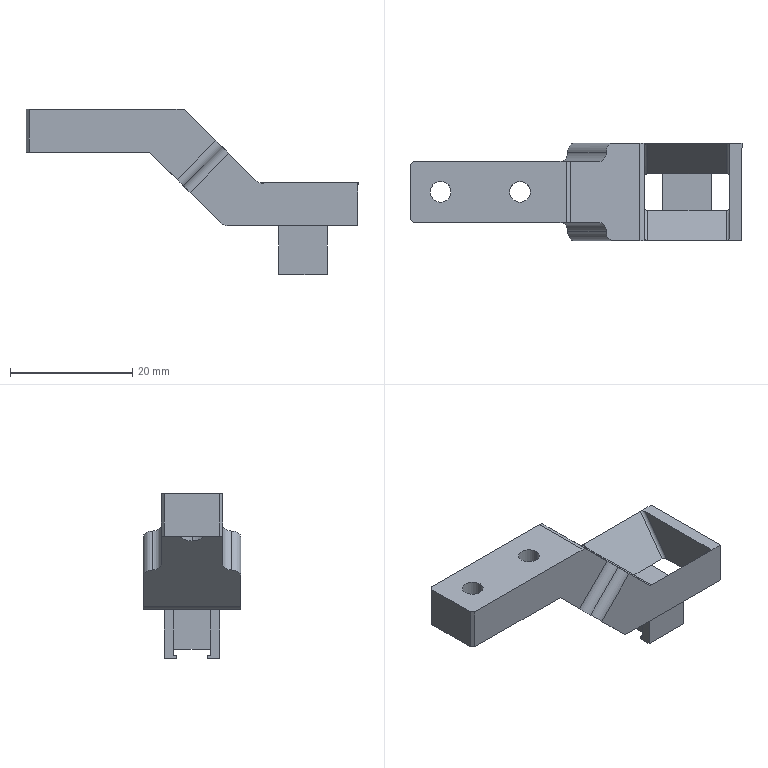NC program | NX | posted with a generic post | part box 54.3 x 16 x 27 mm
Lines 1 to 2092 of 2256, first 1710 of 2082 lines:
N10 G17 G21 G94 G90
(FLOOR_WALL_COPY , TOOL : D63)
N12 T01 M6
N14 G54
N16 G17 G0 G90 X61.65 Y0. S6500 M3
N18 G43 Z30. H1
N20 Z5.
N22 G94 G1 Z2. F1250.
N24 X58.65
N26 X-58.65
N28 X-61.65
N30 Z5.
N32 G0 Z30.
N34 X61.65
N36 Z4.
N38 G1 Z1.
N40 X58.65
N42 X-58.65
N44 X-61.65
N46 Z4.
N48 G0 Z30.
N50 X61.65
N52 Z3.
N54 G1 Z0.
N56 X58.65
N58 X-58.65
N60 X-61.65
N62 Z3.
N64 G0 Z30.
N66 M5
(ADAPTIVE_MILLING_COPY , TOOL : D10)
N68 T10 M6
N70 G54
N72 G17 G0 G90 X-34.694 Y5.359 S9500 M3
N74 G43 Z30. H10
N76 Z-19.
N78 G94 G1 Z-20. F1000.
N80 X-33.303 Y5.066 F3000.
N82 G3 X-32.119 Y5.793 R1.015
N84 G2 X-30.91 Y8.416 R7.757
N86 X-26.126 Y11.331 R8.866
N88 X-19.787 Y12.096 R28.107
N90 X-3.589 Y12.207 R872.404
N92 X-1.666 Y12.973 R40.193
N94 G3 X-1.294 Y14.73 R1.002
N96 X-2.022 Y14.954 Z-19.961 R1.2
N98 G1 X-3.242 Y15.048 Z-19.9
N100 X-5.564 Y15.223
N102 X-18.689
N104 G3 X-27.308 Y14.162 R35.782
N106 G1 X-29.988 Y13.492
N108 G3 X-32.384 Y11.72 R3.927
N110 G1 X-33.273 Y10.231
N112 X-33.344 Y9.998
N114 X-33.595 Y8.591
N116 X-33.946 Y6.622 Z-20.
N118 G3 X-32.052 Y5.992 R1.001
N120 G1 X-31.586 Y7.089
N122 X-31.512 Y7.213
N124 G2 X-29.711 Y9.133 R10.188
N126 X-27.095 Y10.189 R7.286
N128 X-18.08 Y11.276 R40.593
N130 X-5.381 Y11.398 R731.827
N132 G3 X-4.212 Y11.674 R2.037
N134 G1 X-3.221 Y12.351
N136 G3 X-2.96 Y13.916 R1.104
N138 X-4.038 Y14.346 Z-19.939 R1.126
N140 G1 X-4.815 Y14.276 Z-19.9
N142 X-22.927 Y12.645
N144 X-24.919 Y12.466 Z-20.
N146 X-28.102 Y12.179
N148 G3 X-27.771 Y10.008 R-1.1
N150 G2 X-24.571 Y10.157 R20.137
N152 X-7.279 Y10.583 R306.496
N154 G3 X-5.015 Y10.897 R6.389
N156 X-4.229 Y11.659 R4.398
N158 X-4.031 Y13.088 R1.106
N160 X-5.114 Y13.579 Z-19.937 R1.124
N162 G1 X-5.858 Y13.533 Z-19.9
N164 X-20.163 Y12.646
N166 X-22.16 Y12.522 Z-20.
N168 X-25.039 Y12.343
N170 G3 X-24.971 Y10.145 R1.1
N172 G1 X-6.671 Y10.15
N174 X-6.571 Y10.152
N176 X-6.471 Y10.156
N178 X-6.371 Y10.162
N180 X-6.271 Y10.171
N182 G3 X-5.5 Y10.363 R3.095
N184 X-6.169 Y12.398 R1.101
N186 G1 X-6.941 Y12.316
N188 G3 X-6.671 Y10.15 R1.1
N190 X-5.187 Y10.618 R1.697
N192 G1 X-4.784 Y11.062
N194 G3 X-4.802 Y12.436 R1.015
N196 G1 X-5.859 Y13.547
N198 Z-17.
N200 G0 Z30.
N202 X-1.019 Y-15.568
N204 Z-19.
N206 G1 Z-20. F1000.
N208 X-0.945 Y-14.723 F3000.
N210 X-0.895 Y-13.875
N212 G3 X-1.673 Y-12.97 R1.017
N214 X-5.422 Y-12.354 R12.902
N216 X-17.32 Y-12.208 R274.583
N218 G2 X-25.019 Y-12.171 R212.132
N220 X-28.946 Y-9.646 R5.945
N222 G3 X-29.801 Y-9.066 R5.743
N224 G2 X-31.587 Y-7.088 R10.217
N226 G1 X-32.091 Y-5.9
N228 X-32.128 Y-5.76
N230 G3 X-34.083 Y-6.168 R1.
N232 G1 X-34.065 Y-6.286
N234 X-33.768 Y-8.264 Z-19.9
N236 X-33.664 Y-8.985
N238 X-33.539 Y-9.703
N240 X-33.437 Y-9.918
N242 X-33.293 Y-10.107
N244 X-31.166 Y-12.22
N246 G3 X-27.018 Y-14.768 R12.966
N248 X-25.001 Y-15.159 R7.211
N250 G1 X-5.151 Y-16.046
N252 X-4.921 Y-16.026
N254 X-4.7 Y-15.961
N256 X-2.947 Y-15.181
N258 X-2.346 Y-14.919 Z-19.933
N260 X-1.755 Y-14.634 Z-19.966
N262 G3 X-1.354 Y-14.092 Z-20. R1.039
N264 X-1.969 Y-12.864 R1.005
N266 X-4.395 Y-12.014 R21.801
N268 X-10.463 Y-11.485 R33.858
N270 G1 X-11.163 Y-11.47
N272 X-11.963 Y-11.456
N274 X-12.863 Y-11.445
N276 X-13.963 Y-11.436
N278 X-15.363 Y-11.428
N280 X-17.163 Y-11.422
N282 X-19.863 Y-11.418
N284 X-21.663 Y-11.416
N286 X-21.863 Y-11.414
N288 X-22.062 Y-11.407
N290 X-22.162 Y-11.401
N292 X-22.262 Y-11.394
N294 X-22.362 Y-11.386
N296 G2 X-26.048 Y-10.189 R10.868
N298 G1 X-26.145 Y-10.164
N300 X-26.244 Y-10.148
N302 X-26.273 Y-10.145
N304 X-26.571
N306 X-26.626 Y-10.142
N308 X-27.663 Y-10.031
N310 X-27.771 Y-10.008
N312 G2 X-29.181 Y-9.443 R5.526
N314 G3 X-29.862 Y-11.485 R-1.1
N316 G1 X-21.677 Y-12.417
N318 X-19.69 Y-12.644 Z-19.9
N320 X-4.721 Y-14.349
N322 X-4.174 Y-14.415 Z-19.928
N324 X-3.625 Y-14.459 Z-19.955
N326 G3 X-2.842 Y-14.073 Z-20. R1.127
N328 X-3.067 Y-12.447 R1.103
N330 X-6.588 Y-11.131 R7.515
N332 X-14.667 Y-10.662 R58.746
N334 G2 X-20.565 Y-10.571 R130.429
N336 X-22.98 Y-10.146 R25.993
N338 G1 X-26.28 Y-10.145
N340 G3 X-26.366 Y-12.342 R1.1
N342 G1 X-24.497 Y-12.488
N344 X-22.503 Y-12.644 Z-19.9
N346 X-5.256 Y-13.996
N348 X-4.712 Y-14.042 Z-19.927
N350 X-4.166 Y-14.066 Z-19.955
N352 G3 X-3.392 Y-13.645 Z-20. R1.127
N354 X-3.648 Y-12.057 R1.104
N356 X-7.522 Y-10.439 R7.948
N358 G1 X-7.817 Y-10.387
N360 X-8.015 Y-10.355
N362 X-8.312 Y-10.311
N364 X-8.609 Y-10.27
N366 X-8.906 Y-10.233
N368 X-9.205 Y-10.198
N370 X-9.503 Y-10.167
N372 X-9.693 Y-10.149
N374 X-22.993 Y-10.146
N376 G3 X-23.067 Y-12.343 R1.1
N378 G1 X-20.592 Y-12.511
N380 X-18.596 Y-12.646 Z-19.9
N382 X-5.928 Y-13.502
N384 X-4.895 Y-13.56 Z-19.952
N386 G3 X-4.083 Y-13.098 Z-20. R1.117
N388 X-4.263 Y-11.63 R1.106
N390 X-6.784 Y-10.15 R4.657
N392 G1 X-9.784 Y-10.149
N394 G3 X-9.982 Y-12.331 R1.1
N396 G1 X-5.563 Y-13.141
N398 G3 X-4.552 Y-11.318 R1.101
N400 X-5.819 Y-10.211 R3.706
N402 G1 X-5.916 Y-10.184
N404 G3 X-6.916 Y-11.916 R1.418
N406 G1 Z-17.
N408 G0 Z30.
N410 X-6.091 Y-12.459
N412 Z-19.
N414 G1 Z-20. F1000.
N416 G3 X-5.091 Y-10.727 R1.068 F3000.
N418 X-6.174 Y-10.15 R1.435
N420 G1 X-6.874
N422 G3 X-7.874 Y-11.018 R1.015
N424 G1 X-8.105 Y-12.649
N426 Z-17.
N428 G0 Z30.
N430 X-6.845 Y-12.646
N432 Z-18.85
N434 G1 Z-19.85 F1000.
N436 X-6.621 Y-11.939 F3000.
N438 X-6.419 Y-11.227
N440 G3 X-7.293 Y-10.082 R1.014
N442 G2 X-9.133 Y-9.716 R13.216
N444 G3 X-15.616 Y-9.336 R44.907
N446 G1 X-16.615 Y-9.326
N448 X-17.715 Y-9.319
N450 X-19.415 Y-9.312
N452 X-21.715 Y-9.307
N454 X-23.815 Y-9.305
N456 X-24.115 Y-9.303
N458 X-24.315 Y-9.296
N460 X-24.515 Y-9.284
N462 X-24.615 Y-9.277
N464 G2 X-29.165 Y-6.37 R6.019
N466 X-30.957 Y-0.905 R12.945
N468 X-31.153 Y2.882 R17.934
N470 X-28.239 Y7.11 R6.115
N472 X-22.771 Y8.898 R13.157
N474 X-13.784 Y9.273 R80.836
N476 G3 X-9.687 Y9.319 R120.043
N478 G1 X-9.591 Y9.346
N480 X-9.497 Y9.381
N482 X-9.456 Y9.392
N484 X-9.406 Y9.429
N486 X-9.288 Y9.497
N488 X-8.163 Y9.955
N490 X-8.031 Y9.99
N492 X-7.336 Y10.077
N494 G3 X-7.266 Y12.05 R1.
N496 G1 X-9.26 Y12.195 Z-19.75
N498 X-11.233 Y12.327
N500 X-15.116 Y12.331
N502 X-18.998 Y12.315
N504 G3 X-24.303 Y11.742 R33.616
N506 G1 X-26.55 Y11.302
N508 G3 X-28.997 Y10.23 R8.544
N510 X-31.394 Y8.505 R21.965
N512 X-33.33 Y5.962 R7.81
N514 G1 X-34.047 Y4.412
N516 G3 X-34.505 Y1.269 R7.014
N518 X-33.857 Y-2.409 R21.764
N520 G1 X-33.058 Y-5.333
N522 G3 X-30.706 Y-9.442 R10.958
N524 X-27.868 Y-11.569 R11.21
N526 X-26.314 Y-12.061 R5.955
N528 G1 X-25.081 Y-12.23
N530 X-23.842 Y-12.343
N532 X-11.345 Y-13.137
N534 X-11.1 Y-13.119
N536 X-10.864 Y-13.048
N538 X-9.157 Y-12.264
N540 X-8.56 Y-11.996 Z-19.783
N542 X-7.973 Y-11.705 Z-19.816
N544 G3 X-7.579 Y-11.156 Z-19.85 R1.038
N546 X-8.163 Y-9.955 R1.005
N548 X-13.399 Y-8.727 R13.553
N550 X-22.095 Y-8.506 R179.279
N552 G2 X-28.226 Y-4.551 R7.728
N554 X-29.75 Y0.157 R9.996
N556 X-26.545 Y5.851 R6.994
N558 X-20.571 Y7.982 R13.882
N560 X-11.791 Y8.465 R72.135
N562 G3 X-10.334 Y8.726 R3.136
N564 G1 X-9.406 Y9.429
N566 G3 X-9.152 Y10.739 R1.005
N568 X-10.056 Y11.242 Z-19.796 R1.108
N570 G1 X-10.969 Y11.367 Z-19.75
N572 X-12.135 Y11.531
N574 X-13.303 Y11.679
N576 X-15.926 Y11.667
N578 G3 X-18.902 Y11.368 R23.497
N580 G1 X-21.305 Y10.971
N582 X-23.704 Y10.548
N584 G3 X-26.891 Y9.188 R10.193
N586 G1 X-27.71 Y8.621
N588 X-29.561 Y7.204
N590 G3 X-32.73 Y1.225 R9.176
N592 X-32.814 Y-1.042 R10.047
N594 X-31.855 Y-4.187 R8.525
N596 G1 X-31.089 Y-5.624
N598 X-30.306 Y-7.053
N600 G3 X-23.608 Y-11.372 R9.088
N602 G1 X-12.47 Y-12.679
N604 G3 X-11.896 Y-12.575 R1.05
N606 G1 X-10.355 Y-11.784
N608 X-9.763 Y-11.486 Z-19.783
N610 X-9.183 Y-11.166 Z-19.816
N612 G3 X-8.815 Y-10.617 Z-19.85 R1.04
N614 X-9.288 Y-9.497 R1.007
N616 X-12.559 Y-8.256 R7.076
N618 X-19.736 Y-7.767 R53.459
N620 G2 X-27.173 Y-3.154 R8.398
N622 X-25.88 Y3.62 R6.296
N624 X-20.28 Y6.732 R11.07
N626 X-13.542 Y7.556 R35.54
N628 G3 X-11.086 Y7.954 R8.006
N630 X-10.374 Y8.695 R3.575
N632 G1 X-10.294 Y8.756
N634 G3 X-10.025 Y10.039 R1.005
N636 X-10.85 Y10.556 Z-19.799 R1.036
N638 G1 X-11.825 Y10.7 Z-19.75
N640 X-12.933 Y10.87
N642 X-14.044 Y11.017
N644 X-14.191 Y11.006
N646 X-16.725 Y10.629
N648 X-19.255 Y10.231
N650 G3 X-23.855 Y8.721 R17.997
N652 G1 X-24.674 Y8.275
N654 X-25.468 Y7.786
N656 X-26.937 Y6.791
N658 G3 X-30.071 Y2.932 R9.819
N660 X-30.036 Y-4.241 R8.823
N662 X-29.08 Y-5.809 R8.521
N664 G1 X-28.315 Y-6.794
N666 X-27.518 Y-7.754
N668 G3 X-26.567 Y-8.544 R4.338
N670 G1 X-25.038 Y-9.453
N672 G3 X-22.043 Y-10.464 R9.838
N674 X-16.476 Y-11.211 R83.227
N676 G1 X-13.423 Y-11.502
N678 X-11.236 Y-11.196
N680 X-10.586 Y-11.109 Z-19.783
N682 X-9.94 Y-10.996 Z-19.816
N684 G3 X-9.407 Y-10.583 Z-19.85 R1.038
N686 X-9.645 Y-9.248 R1.005
N688 X-13.45 Y-7.57 R7.472
N690 X-18.618 Y-7.024 R54.385
N692 G2 X-23.16 Y-5.362 R8.744
N694 X-24.483 Y0.921 R5.298
N696 X-19.901 Y5.169 R8.486
N698 X-14.187 Y6.563 R22.236
N700 G3 X-11.583 Y7.227 R8.616
N702 X-10.787 Y8.193 R5.823
N704 X-10.704 Y9.294 R1.01
N706 X-11.429 Y9.8 Z-19.804 R1.05
N708 G1 X-12.482 Y10.065 Z-19.75
N710 X-13.363 Y10.291
N712 X-14.248 Y10.497
N714 X-14.468 Y10.491
N716 X-14.684 Y10.443
N718 G3 X-22.166 Y7.516 R103.306
N720 X-25.649 Y4.921 R11.193
N722 G1 X-26.749 Y3.678
N724 G3 X-27.894 Y1.069 R6.093
N726 X-28.036 Y-0.574 R8.104
N728 G1 X-27.976 Y-2.854
N730 G3 X-26.964 Y-5.913 R6.857
N732 X-25.992 Y-7.277 R8.317
N734 X-23.817 Y-8.745 R6.341
N736 G1 X-23.236 Y-8.958
N738 X-22.642 Y-9.13
N740 X-19.924 Y-9.778
N742 X-17.197 Y-10.386
N744 X-14.149 Y-10.961
N746 X-13.905 Y-10.946
N748 X-12.025 Y-10.599
N750 X-11.376 Y-10.484 Z-19.783
N752 X-10.731 Y-10.345 Z-19.816
N754 G3 X-10.218 Y-9.918 Z-19.85 R1.039
N756 X-10.374 Y-8.695 R1.007
N758 X-12.862 Y-7.221 R4.942
N760 X-17.477 Y-6.363 R33.121
N762 G2 X-20.725 Y-4.615 R4.609
N764 X-20.867 Y0.792 R5.115
N766 X-16.551 Y4.507 R8.832
N768 X-12.634 Y6.02 R423.42
N770 G3 X-11.582 Y6.817 R2.166
N772 G1 X-11.285 Y7.522
N774 X-11.235 Y7.609
N776 G3 X-11.352 Y8.781 R1.007
N778 X-12.261 Y9.105 Z-19.8 R1.037
N780 G1 X-13.254 Y9.042 Z-19.75
N782 X-15.116 Y8.923
N784 X-15.357 Y8.874
N786 X-15.581 Y8.773
N788 X-17.753 Y7.422
N790 X-19.916 Y6.056
N792 G3 X-22.572 Y3.943 R20.484
N794 X-24.39 Y0.271 R6.692
N796 X-24.365 Y-2.478 R8.177
N798 G1 X-24.214 Y-3.297
N800 X-24.013 Y-4.106
N802 G3 X-21.836 Y-7.454 R7.439
N804 X-18.412 Y-9.447 R9.742
N806 G1 X-14.43 Y-10.771
N808 G3 X-13.875 Y-10.793 R1.056
N810 G1 X-12.245 Y-10.391
N812 X-11.585 Y-10.233 Z-19.784
N814 X-10.931 Y-10.054 Z-19.818
N816 G3 X-10.457 Y-9.636 Z-19.85 R1.043
N818 X-10.532 Y-8.521 R1.01
N820 X-13.175 Y-6.65 R4.905
N822 G2 X-15.373 Y-5.98 R58.857
N824 X-17.484 Y-2.276 R3.983
N826 X-15.357 Y2.44 R6.994
N828 X-12.432 Y5.015 R49.357
N830 G3 X-11.793 Y6.271 R1.565
N832 G1 X-11.757 Y6.403
N834 X-11.563 Y6.864
N836 G3 X-11.966 Y8.107 R1.005
N838 X-12.933 Y8.151 Z-19.8 R1.037
N840 G1 X-13.86 Y7.798 Z-19.75
N842 X-14.853 Y7.423
N844 X-15.839 Y7.032
N846 X-16.063 Y6.864
N848 G3 X-17.105 Y5.709 R8.737
N850 G1 X-19.588 Y1.735
N852 G3 X-20.191 Y-2.998 R5.721
N854 G1 X-19.089 Y-6.475
N856 G3 X-16.905 Y-8.674 R3.401
N858 G1 X-15.155 Y-9.236
N860 X-12.948 Y-9.513
N862 X-12.296 Y-9.598 Z-19.783
N864 X-11.642 Y-9.659 Z-19.816
N866 G3 X-11.021 Y-9.403 Z-19.85 R1.039
N868 X-10.9 Y-8.047 R1.005
N870 X-12.642 Y-6.405 R5.646
N872 G2 X-14.353 Y-1.433 R5.328
N874 X-12.841 Y2.456 R10.733
N876 G3 X-11.994 Y4.04 R11.478
N878 G2 X-11.854 Y5.828 R15.376
N880 G3 X-13.091 Y6.934 R1.002
N882 X-13.775 Y6.381 Z-19.805 R1.172
N884 G1 X-14.41 Y5.487 Z-19.75
N886 X-15.672 Y3.71
N888 X-16.221 Y2.643
N890 X-16.718 Y1.551
N892 X-16.971 Y0.848
N894 X-17.186 Y0.133
N896 X-17.485 Y-0.991
N898 X-17.762 Y-2.12
N900 G3 X-16.984 Y-5.781 R4.962
N902 G1 X-15.716 Y-7.64
N904 G3 X-15.245 Y-8.012 R1.047
N906 G1 X-13.515 Y-8.669
N908 X-12.898 Y-8.909 Z-19.783
N910 X-12.273 Y-9.126 Z-19.816
N912 G3 X-11.617 Y-9.032 Z-19.85 R1.039
N914 X-11.216 Y-7.64 R1.004
N916 G2 X-12.271 Y-5.56 R22.33
N918 X-12.263 Y0.337 R9.427
N920 G3 X-11.942 Y1.595 R8.724
N922 G1 X-11.965 Y1.841
N924 X-11.968 Y1.891
N926 Y4.191
N928 G3 X-14.166 Y4.127 R-1.1
N930 G1 X-13.475 Y-7.829
N932 G3 X-11.363 Y-7.338 R-1.1
N934 G2 X-11.968 Y-4.964 R5.796
N936 X-11.891 Y-1.077 R35.506
N938 G3 X-11.706 Y0.223 R3.713
N940 G2 X-11.943 Y1.604 R11.623
N942 G3 X-12.978 Y2.517 R1.015
N944 G1 X-14.466 Y2.474
N946 Z-16.85
N948 G0 Z30.
N950 X-6.75 Y-12.611
N952 Z-17.806
N954 G1 Z-18.806 F1000.
N956 X-6.24 Y-12.163 F3000.
N958 X-5.748 Y-11.697
N960 G3 X-6.358 Y-10.076 R1.012
N962 G2 X-9.516 Y-8.488 R5.316
N964 X-10.937 Y-4.864 R5.696
N966 G1 X-10.942 Y-1.135
N968 G2 X-11.024 Y2.961 R35.702
N970 G3 X-10.926 Y5.036 R9.258
N972 G2 X-9.424 Y8.584 R5.579
N974 X-6.327 Y10.081 R5.365
N976 G3 X-5.89 Y11.852 R1.001
N978 X-6.511 Y12.083 Z-18.773 R1.287
N980 G1 X-7.818 Y12.325 Z-18.706
N982 X-8.654 Y12.487
N984 X-9.495 Y12.624
N986 G3 X-10.225 Y12.331 R1.026
N988 G1 X-11.236 Y11.324
N990 X-12.234 Y10.304
N992 G3 X-13.245 Y8.492 R5.115
N994 X-14.022 Y5.095 R21.177
N996 G1 X-14.086 Y4.351
N998 X-14.113 Y3.604
N1000 X-14.106 Y-1.9
N1002 X-14.05 Y-2.13
N1004 X-13.436 Y-3.783
N1006 X-12.819 Y-5.424 Z-18.794
N1008 X-12.68 Y-5.626 Z-18.806
N1010 G3 X-10.931 Y-4.963 R1.001
N1012 G1 Y3.565
N1014 G3 X-11.79 Y4.564 R1.016
N1016 G1 X-13.431 Y4.812
N1018 Z-15.806
N1020 G0 Z30.
N1022 X-6.587 Y-12.792
N1024 Z-17.21
N1026 G1 Z-18.21 F1000.
N1028 X-5.56 Y-11.727 F3000.
N1030 G3 X-5.977 Y-10.065 R1.012
N1032 G2 X-9.785 Y-7.279 R5.357
N1034 X-10.331 Y-4.968 R6.009
N1036 G1 Y4.986
N1038 X-10.327 Y5.048
N1040 G2 X-6.07 Y10.028 R5.166
N1042 G1 X-6.013 Y10.046
N1044 X-5.918 Y10.078
N1046 G3 X-5.517 Y11.732 R1.012
N1048 G1 X-6.567 Y12.829
N1050 Z-15.21
N1052 G0 Z30.
N1054 X-7.115 Y-11.501
N1056 Z-16.613
N1058 G1 Z-17.613 F1000.
N1060 G3 X-5.701 Y-10.087 R1.04 F3000.
N1062 G1 X-5.846 Y-10.004
N1064 X-7.12 Y-9.453
N1066 X-7.233 Y-9.387
N1068 G2 X-9.565 Y-6.254 R5.44
N1070 G1 X-9.726 Y-5.034
N1072 X-9.731 Y-4.965
N1074 Y4.965
N1076 X-9.726 Y5.035
N1078 G2 X-8.175 Y8.66 R5.519
N1080 X-5.92 Y9.979 R6.444
N1082 G3 X-5.777 Y11.756 R1.012
N1084 G1 X-6.896 Y12.473
N1086 Z-14.613
N1088 G0 Z30.
N1090 X-7.005 Y-11.472
N1092 Z-16.016
N1094 G1 Z-17.016 F1000.
N1096 G3 X-5.591 Y-10.058 R1.099 F3000.
N1098 X-6.976 Y-9.168 R6.404
N1100 G2 X-9.131 Y-4.969 R5.359
N1102 G1 Y4.969
N1104 X-9.127 Y5.031
N1106 G2 X-6.983 Y9.161 R5.307
N1108 G3 X-5.612 Y10.033 R6.372
N1110 G1 X-5.55 Y10.111
N1112 G3 X-5.698 Y11.511 R1.005
N1114 X-6.582 Y11.723 Z-16.969 R1.152
N1116 G1 X-7.644 Y11.661 Z-16.916
N1118 X-8.519 Y11.613
N1120 X-9.392 Y11.547
N1122 G3 X-9.897 Y11.275 R1.051
N1124 G1 X-10.293 Y10.881
N1126 X-10.657 Y10.458
N1128 X-10.849 Y10.143
N1130 X-11.009 Y9.81
N1132 X-11.776 Y7.82
N1134 G3 X-12.397 Y4.064 R11.823
N1136 G1 Y-7.022
N1138 G3 X-11.201 Y-9.937 R4.172
N1140 G1 X-10.556 Y-10.597
N1142 X-9.898 Y-11.244
N1144 G3 X-9.37 Y-11.444 R1.053
N1146 G1 X-7.879 Y-11.558
N1148 X-7.099 Y-11.62 Z-16.955
N1150 X-6.319 Y-11.666 Z-16.994
N1152 X-6.106 Y-11.624 Z-17.005
N1154 X-5.904 Y-11.544 Z-17.016
N1156 G3 X-5.802 Y-9.861 R1.001
N1158 X-7.331 Y-10.313 R1.013
N1160 G1 X-7.825 Y-11.573
N1162 Z-14.016
N1164 G0 Z30.
N1166 X-6.988 Y-12.335
N1168 Z-15.419
N1170 G1 Z-16.419 F1000.
N1172 X-5.798 Y-11.155 F3000.
N1174 G3 X-5.639 Y-9.925 R1.017
N1176 G1 X-5.69 Y-9.839
N1178 X-5.928 Y-9.517
N1180 X-5.994 Y-9.442
N1182 X-6.031 Y-9.405
N1184 G2 X-7.901 Y-7.438 R6.188
N1186 X-8.53 Y-4.966 R5.993
N1188 G1 Y4.966
N1190 X-8.526 Y5.034
N1192 G2 X-7.042 Y8.594 R5.493
N1194 G3 X-5.764 Y9.712 R7.285
N1196 G1 X-5.561 Y10.057
N1198 G3 X-5.997 Y11.469 R1.004
N1200 X-6.929 Y11.447 Z-16.371 R1.136
N1202 G1 X-7.908 Y11.106 Z-16.319
N1204 X-8.776 Y10.811
N1206 X-9.636 Y10.493
N1208 G3 X-10.061 Y10.057 R1.046
N1210 G1 X-10.794 Y8.565
N1212 G3 X-11.328 Y6.58 R7.405
N1214 X-11.699 Y2.357 R43.65
N1216 G1 X-11.709 Y1.359
N1218 X-11.698 Y0.362
N1220 X-11.514 Y-5.672
N1222 G3 X-10.803 Y-8.558 R7.18
N1224 G1 X-10.442 Y-9.314
N1226 X-10.059 Y-10.06
N1228 G3 X-9.566 Y-10.433 R1.044
N1230 G1 X-8.172 Y-10.914
N1232 X-7.432 Y-11.172 Z-16.359
N1234 X-6.687 Y-11.415 Z-16.398
N1236 X-6.472 Y-11.428 Z-16.409
N1238 X-6.258 Y-11.402 Z-16.419
N1240 G3 X-5.639 Y-9.925 R1.003
N1242 X-6.096 Y-9.352 R2.019
N1244 X-7.563 Y-9.571 R1.014
N1246 G1 X-8.362 Y-10.743
N1248 Z-13.419
N1250 G0 Z30.
N1252 X-7.5 Y-11.654
N1254 Z-14.823
N1256 G1 Z-15.823 F1000.
N1258 X-6.775 Y-11.153 F3000.
N1260 X-6.064 Y-10.632
N1262 G3 X-5.874 Y-9.437 R1.017
N1264 X-7.16 Y-7.676 R9.203
N1266 G2 X-7.93 Y-4.968 R5.773
N1268 G1 Y4.963
N1270 X-7.925 Y5.035
N1272 G2 X-7.198 Y7.612 R5.88
N1274 G1 X-7.119 Y7.738
N1276 X-6.213 Y8.808
N1278 X-6.075 Y9.017
N1280 X-5.807 Y9.554
N1282 G3 X-6.093 Y10.805 R1.017
N1284 G1 X-7.375 Y11.794
N1286 Z-12.823
N1288 G0 Z30.
N1290 X-7.908 Y-10.894
N1292 Z-14.226
N1294 G1 Z-15.226 F1000.
N1296 X-7.151 Y-10.491 F3000.
N1298 X-6.407 Y-10.067
N1300 G3 X-6.08 Y-8.904 R1.017
N1302 X-6.985 Y-6.883 R17.907
N1304 G2 X-7.33 Y-5.008 R6.062
N1306 G1 Y5.002
N1308 X-7.328 Y5.047
N1310 G2 X-6.507 Y7.86 R5.576
N1312 G1 X-6.05 Y8.969
N1314 G3 X-6.497 Y10.239 R1.015
N1316 G1 X-7.867 Y10.993
N1318 Z-12.226
N1320 G0 Z30.
N1322 X-8.312 Y-10.058
N1324 Z-13.629
N1326 G1 Z-14.629 F1000.
N1328 X-7.501 Y-9.72 F3000.
N1330 X-6.698 Y-9.36
N1332 G3 X-6.246 Y-8.28 R1.017
N1334 G2 X-6.73 Y-5.547 R12.969
N1336 G1 Y5.537
N1338 X-6.729 Y5.569
N1340 X-6.682 Y6.348
N1342 X-6.67 Y6.432
N1344 X-6.254 Y8.285
N1346 G3 X-6.848 Y9.438 R1.016
N1348 G1 X-8.3 Y10.049
N1350 Z-11.629
N1352 G0 Z30.
N1354 X-7.877 Y-10.822
N1356 Z-13.032
N1358 G1 Z-14.032 F1000.
N1360 X-7.101 Y-10.473 F3000.
N1362 X-6.336 Y-10.102
N1364 G3 X-5.927 Y-8.978 R1.017
N1366 G2 X-6.13 Y-7.667 R5.504
N1368 G1 Y7.567
N1370 X-6.124 Y7.644
N1372 G2 X-5.633 Y9.677 R5.744
N1374 G3 X-6.066 Y10.944 R1.015
N1376 G1 X-7.406 Y11.706
N1378 Z-11.032
N1380 G0 Z30.
N1382 X-2.901 Y-15.133
N1384 Z-12.435
N1386 G1 Z-13.435 F1000.
N1388 X-2.615 Y-14.332 F3000.
N1390 X-2.351 Y-13.524
N1392 G3 X-2.856 Y-12.458 R1.017
N1394 G2 X-5.333 Y-9.28 R5.587
N1396 G1 X-5.524 Y-8.029
N1398 X-5.53 Y-7.95
N1400 Y7.954
N1402 X-5.525 Y8.026
N1404 G2 X-4.026 Y11.598 R5.591
N1406 G1 X-3.929 Y11.694
N1408 X-3.052 Y12.358
N1410 G3 X-2.694 Y13.451 R1.02
N1412 G1 X-3.17 Y15.053
N1414 Z-10.435
N1416 G0 Z30.
N1418 X-0.233 Y-15.601
N1420 Z-11.839
N1422 G1 Z-12.839 F1000.
N1424 X-0.527 Y-13.726 F3000.
N1426 G3 X-1.143 Y-12.947 R1.024
N1428 G2 X-4.754 Y-9.271 R5.333
N1430 G1 X-4.925 Y-8.036
N1432 X-4.93 Y-7.964
N1434 Y7.964
N1436 X-4.925 Y8.036
N1438 G2 X-3.433 Y11.599 R5.576
N1440 X-1.124 Y12.955 R5.84
N1442 G3 X-0.514 Y14.085 R1.017
N1444 G1 X-0.796 Y15.525
N1446 Z-9.839
N1448 G0 Z30.
N1450 X0.379 Y-15.603
N1452 Z-11.242
N1454 G1 Z-12.242 F1000.
N1456 X0.082 Y-13.728 F3000.
N1458 G3 X-0.534 Y-12.951 R1.024
N1460 G2 X-3.647 Y-10.522 R5.477
N1462 X-4.329 Y-7.964 R6.077
N1464 G1 Y7.964
N1466 X-4.324 Y8.036
N1468 G2 X-2.833 Y11.599 R5.576
N1470 X-0.524 Y12.955 R5.84
N1472 G3 X0.086 Y14.085 R1.017
N1474 G1 X-0.196 Y15.525
N1476 Z-9.242
N1478 G0 Z30.
N1480 X0.979 Y-15.603
N1482 Z-10.645
N1484 G1 Z-11.645 F1000.
N1486 X0.682 Y-13.728 F3000.
N1488 G3 X0.066 Y-12.951 R1.024
N1490 G2 X-3.046 Y-10.522 R5.477
N1492 X-3.729 Y-7.964 R6.077
N1494 G1 Y7.964
N1496 X-3.724 Y8.036
N1498 G2 X-2.232 Y11.599 R5.576
N1500 X0.076 Y12.955 R5.84
N1502 G3 X0.686 Y14.085 R1.017
N1504 G1 X0.404 Y15.525
N1506 Z-8.645
N1508 G0 Z30.
N1510 X1.579 Y-15.603
N1512 Z-10.048
N1514 G1 Z-11.048 F1000.
N1516 X1.282 Y-13.728 F3000.
N1518 G3 X0.666 Y-12.951 R1.024
N1520 G2 X-2.446 Y-10.522 R5.477
N1522 X-3.129 Y-7.964 R6.077
N1524 G1 Y7.964
N1526 X-3.124 Y8.036
N1528 G2 X-1.632 Y11.599 R5.576
N1530 X0.676 Y12.955 R5.84
N1532 G3 X1.286 Y14.085 R1.017
N1534 G1 X1.004 Y15.525
N1536 Z-8.048
N1538 G0 Z30.
N1540 X2.179 Y-15.603
N1542 Z-9.452
N1544 G1 Z-10.452 F1000.
N1546 X1.882 Y-13.728 F3000.
N1548 G3 X1.266 Y-12.951 R1.024
N1550 G2 X-1.846 Y-10.522 R5.476
N1552 X-2.529 Y-7.964 R6.077
N1554 G1 Y7.964
N1556 X-2.524 Y8.036
N1558 G2 X-1.032 Y11.599 R5.576
N1560 X1.276 Y12.955 R5.84
N1562 G3 X1.886 Y14.085 R1.017
N1564 G1 X1.604 Y15.525
N1566 Z-7.452
N1568 G0 Z30.
N1570 X2.779 Y-15.603
N1572 Z-8.855
N1574 G1 Z-9.855 F1000.
N1576 X2.482 Y-13.728 F3000.
N1578 G3 X1.866 Y-12.951 R1.024
N1580 G2 X-1.246 Y-10.522 R5.476
N1582 X-1.929 Y-7.964 R6.077
N1584 G1 Y7.964
N1586 X-1.924 Y8.036
N1588 G2 X-0.432 Y11.599 R5.576
N1590 X1.876 Y12.955 R5.84
N1592 G3 X2.486 Y14.085 R1.017
N1594 G1 X2.204 Y15.525
N1596 Z-6.855
N1598 G0 Z30.
N1600 X3.379 Y-15.602
N1602 Z-8.258
N1604 G1 Z-9.258 F1000.
N1606 X3.082 Y-13.728 F3000.
N1608 G3 X2.466 Y-12.951 R1.024
N1610 G2 X-0.646 Y-10.522 R5.476
N1612 X-1.329 Y-7.964 R6.077
N1614 G1 Y7.964
N1616 X-1.324 Y8.036
N1618 G2 X0.168 Y11.599 R5.576
N1620 X2.477 Y12.955 R5.84
N1622 G3 X3.087 Y14.085 R1.017
N1624 G1 X2.804 Y15.525
N1626 Z-6.258
N1628 G0 Z30.
N1630 X3.991 Y-15.604
N1632 Z-7.661
N1634 G1 Z-8.661 F1000.
N1636 X3.692 Y-13.726 F3000.
N1638 G3 X3.077 Y-12.951 R1.024
N1640 G2 X-0.04 Y-10.519 R5.508
N1642 X-0.728 Y-7.963 R6.092
N1644 G1 Y7.962
N1646 X-0.723 Y8.037
N1648 G2 X0.878 Y11.683 R5.589
N1650 X3.18 Y12.972 R5.902
N1652 G3 X3.893 Y14.215 R1.014
N1654 G1 X3.531 Y15.538
N1656 Z-5.661
N1658 G0 Z30.
N1660 X4.808 Y-15.604
N1662 Z-7.065
N1664 G1 Z-8.065 F1000.
N1666 X4.5 Y-13.741 F3000.
N1668 G3 X3.872 Y-12.965 R1.024
N1670 G2 X0.686 Y-10.55 R5.553
N1672 X-0.045 Y-7.96 R6.15
N1674 G1 Y7.96
N1676 X-0.039 Y8.039
N1678 G2 X1.528 Y11.631 R5.66
N1680 X3.891 Y12.973 R5.938
N1682 G3 X4.516 Y14.1 R1.017
N1684 G1 X4.246 Y15.536
N1686 Z-5.065
N1688 G0 Z30.
N1690 X34.843 Y0.047
N1692 Z-6.85
N1694 G1 Z-7.85 F1000.
N1696 X33.487 Y0.577 F3000.
N1698 G3 X32.196 Y0.047 R1.015
N1700 X31.553 Y-3.113 R9.424
N1702 G2 X31.34 Y-6.203 R38.076
N1704 X27.988 Y-10.351 R6.416
N1706 X22.236 Y-11.903 R14.818
N1708 X11.743 Y-12.182 R123.888
N1710 X7.145 Y-12.145 R75.284
N1712 X2.888 Y-9.107 R6.187
N1714 X1.149 Y-3.416 R13.65
N1716 X0.874 Y5.872 R74.165
N1718 X3.908 Y10.129 R6.155
N1720 X9.703 Y11.868 R13.787
N1722 X18.293 Y12.174 R89.934
N1724 X24.992 Y12.151 R151.593
N1726 X29.261 Y9.136 R6.138
N1728 X31.041 Y1.946 R13.717
N1730 X30.646 Y-3.837 R58.603
N1732 X26.347 Y-9.315 R8.08
N1734 X19.719 Y-11.063 R17.474
N1736 X9.728 Y-11.329 R99.164
N1738 X3.909 Y-7.385 R7.727
N1740 X1.995 Y-0.914 R15.961
N1742 X1.807 Y3.574 R22.992
N1744 X5.772 Y9.159 R7.678
N1746 X12.059 Y11.004 R16.
N1748 X22.546 Y11.317 R81.759
N1750 X28.358 Y7.199 R7.781
N1752 X29.878 Y1.144 R13.6
N1754 X29.353 Y-3.587 R11.151
N1756 X26.21 Y-7.596 R9.195
N1758 X24.661 Y-8.986 R5.088
N1760 X21.553 Y-9.86 R10.076
N1762 X11.686 Y-10.467 R55.909
N1764 X4.871 Y-5.973 R8.688
N1766 X2.912 Y1.489 R15.252
N1768 X6.989 Y8.005 R8.223
N1770 X13.608 Y10.112 R16.396
N1772 X20.691 Y10.434 R39.602
N1774 X24.445 Y9.076 R8.283
N1776 X26.918 Y6.653 R5.884
N1778 X28.578 Y-0.915 R11.594
N1780 X27.356 Y-4.176 R10.549
N1782 G1 X27.327 Y-4.272
N1784 X27.307 Y-4.369
N1786 X27.3 Y-4.428
N1788 Y-4.466
N1790 X27.296 Y-4.534
N1792 X27.134 Y-5.765
N1794 X27.098 Y-5.897
N1796 X26.636 Y-7.011
N1798 X26.568 Y-7.13
N1800 X26.203 Y-7.606
N1802 X25.98 Y-7.903
N1804 X25.737 Y-8.183
N1806 G2 X23.415 Y-9.484 R5.802
N1808 G1 X22.184 Y-9.646
N1810 X22.116 Y-9.65
N1812 G2 X13.286 Y-9.604 R219.796
N1814 X5.568 Y-4.289 R9.522
N1816 X4.494 Y1.59 R8.787
N1818 X8.944 Y7.337 R8.708
N1820 G3 X10.533 Y8.153 R41.4
N1822 G2 X14.116 Y9.646 R5.53
N1824 G1 X14.184 Y9.65
N1826 X22.116
N1828 X22.184 Y9.646
N1830 G2 X24.47 Y9.065 R5.686
N1832 G3 X25.047 Y9.008 R1.05
N1834 G1 X25.872 Y9.171
N1836 X27.834 Y9.559 Z-7.75
N1838 G2 X28.97 Y9.065 R1.011
N1840 G1 X30.155 Y6.869
N1842 X31.288 Y4.646
N1844 G2 X31.792 Y2.27 R5.192
N1846 X31.56 Y-1.464 R36.335
N1848 X30.807 Y-5.115 R23.206
N1850 X29.321 Y-8.518 R16.678
N1852 G1 X28.508 Y-9.896
N1854 G2 X26.656 Y-11.56 R5.264
N1856 X23.763 Y-12.509 R8.582
N1858 G1 X23.021 Y-12.6
N1860 X22.276 Y-12.653
N1862 X17.366 Y-12.832
N1864 G2 X16.501 Y-12.392 R1.014
N1866 G1 X16.352 Y-12.171
N1868 X15.234 Y-10.513 Z-7.85
N1870 X14.854 Y-9.97
N1872 G3 X14.184 Y-9.65 R1.029
N1874 G2 X10.54 Y-8.226 R5.868
N1876 X6.359 Y-2.869 R11.418
N1878 X8.108 Y4.552 R7.505
N1880 G3 X9.154 Y5.755 R7.65
N1882 G2 X10.537 Y8.158 R5.951
N1884 G3 X9.17 Y9.616 R1.
N1886 G1 X8.92 Y9.396
N1888 X7.418 Y8.075 Z-7.75
N1890 X6.191 Y6.993
N1892 X5.026 Y5.809
N1894 G3 X3.966 Y4.062 R6.153
N1896 X3.073 Y0.918 R12.49
N1898 X4.282 Y-5.765 R11.231
N1900 G1 X4.676 Y-6.458
N1902 X5.108 Y-7.128
N1904 X7.174 Y-10.083
N1906 G3 X7.924 Y-10.507 R1.016
N1908 G1 X9.618 Y-10.624
N1910 X10.307 Y-10.676 Z-7.785
N1912 X10.997 Y-10.708 Z-7.819
N1914 G3 X11.558 Y-10.474 Z-7.85 R1.046
N1916 X11.52 Y-8.918 R1.003
N1918 G2 X9.625 Y-6.961 R5.957
N1920 X7.751 Y-3.012 R11.496
N1922 X8.523 Y2.339 R8.694
N1924 G3 X9. Y3.573 R6.295
N1926 G2 X9.192 Y5.861 R10.267
N1928 G3 X7.031 Y6.094 R-1.1
N1930 G1 X7.681 Y-7.731
N1932 G3 X9.732 Y-7.13 R-1.1
N1934 G2 X8.769 Y-2.998 R9.269
N1936 X9. Y-0.313 R14.799
N1938 G1 Y3.587
N1940 G3 X6.8 Y3.567 R-1.1
N1942 G1 X6.976 Y-5.929
N1944 G3 X9.167 Y-5.765 R-1.1
N1946 G1 X9.005 Y-4.534
N1948 X9. Y-4.466
N1950 Y-0.266
N1952 G3 X8.552 Y0.568 R1.014
N1954 G1 X8.172 Y0.82
N1956 X6.505 Y1.924 Z-7.75
N1958 X6.25 Y2.095
N1960 X6.026 Y2.305
N1962 G2 X5.818 Y2.916 R1.041
N1964 G1 X5.815 Y4.364
N1966 X5.831 Y5.811
N1968 G2 X7.586 Y9.684 R6.061
N1970 X12.476 Y12.541 R10.034
N1972 X15.431 Y12.916 R12.126
N1974 G1 X17.639 Y12.917
N1976 X19.846 Y12.901
N1978 G2 X22.743 Y12.675 R34.677
N1980 G1 X24.669 Y12.434
N1982 G2 X25.548 Y11.352 R1.024
N1984 G1 X25.607 Y9.353 Z-7.85
N1986 X25.644 Y8.511
N1988 X25.717 Y8.289
N1990 X25.834 Y8.087
N1992 G2 X27.16 Y5.566 R5.483
N1994 X27.586 Y1.099 R18.633
N1996 X27.3 Y-0.831 R38.01
N1998 G1 Y-4.431
N2000 G3 X29.5 Y-4.414 R-1.1
N2002 G1 X29.35 Y5.726
N2004 G3 X27.16 Y5.566 R-1.1
N2006 G1 X27.296 Y4.534
N2008 X27.3 Y4.466
N2010 Y-0.834
N2012 G3 X27.506 Y-1.445 R1.052
N2014 G1 X29.8 Y-4.466
N2016 Z-4.85
N2018 G0 Z30.
N2020 M5
(FLOOR_WALL_1_1 , TOOL : D6)
N2022 T06 M6
N2024 G54
N2026 G17 G0 G90 X31.145 Y-12.123 S9500 M3
N2028 G43 Z30. H6
N2030 Z-6.5
N2032 G94 G1 Z-8. F1250.
N2034 X30.67 Y-11.3
N2036 G3 X30.15 Y-11. R0.6
N2038 G1 X2.768
N2040 Y-8.233
N2042 X30.15
N2044 Y-5.467
N2046 X25.45
N2048 Y-2.7
N2050 X30.15
N2052 Y0.067
N2054 X25.45
N2056 Y2.833
N2058 X30.15
N2060 Y5.6
N2062 X25.45
N2064 G3 X25.75 Y5.08 R0.6
N2066 G1 Z-6.5
N2068 G0 Z30.
N2070 X25.45 Y-5.467
N2072 Z-6.5
N2074 G1 Z-8.
N2076 Y-7.5
N2078 G2 X25.15 Y-7.8 R0.3
N2080 G1 X11.15
N2082 G2 X10.85 Y-7.5 R0.3
N2084 G1 Y-5.467
N2086 X2.768
N2088 Y-2.7
N2090 X10.85
N2092 Y0.067
N2094 X2.768
N2096 Y2.833
N2098 X10.85
N2100 Y5.6
N2102 X2.768
N2104 Y8.366
N2106 X30.15
N2108 G2 X30.67 Y8.066 R0.6
N2110 G1 X25.45 Y8.02
N2112 G3 X25.15 Y7.5 R0.6
N2114 G1 Y-7.5
N2116 X11.15
N2118 Y7.5
N2120 X25.15
N2122 G3 X25.67 Y7.8 R0.6
N2124 G1 X26.297 Y8.887
N2126 Z-6.5
N2128 G0 Z30.
N2130 X-31.273 Y-6.737
N2132 Z-18.5
N2134 G1 Z-20.
N2136 X-30.45 Y-6.262
N2138 G3 X-30.15 Y-5.743 R0.6
N2140 G1 Y5.743
N2142 X-27.893 Y8.
N2144 X-27.303
N2146 Y-8.
N2148 X-24.455
N2150 Y8.
N2152 X-21.608
N2154 Y-8.
N2156 X-18.761
N2158 Y8.
N2160 X-15.913
N2162 Y-8.
N2164 X-13.066
N2166 Y8.
N2168 X-10.219
N2170 Y-8.
N2172 G2 X-10.519 Y-8.52 R0.6
N2174 G1 X-12.217 Y-9.5
N2176 Z-18.5
N2178 G0 Z30.
N2180 X-11.917
N2182 Z-18.5
N2184 G1 Z-20.
N2186 X-10.219 Y-8.52
N2188 G3 X-9.919 Y-8. R0.6
N2190 G1 Y-2.005
N2192 G2 X-9.15 Y0. R3.
N2194 X-9.919 Y2.005 R3.
N2196 G1 Y8.
N2198 G3 X-10.219 Y8.52 R0.6
N2200 G1 X-11.917 Y9.5
N2202 Z-18.5
N2204 G0 Z30.
N2206 M5
(ZLEVEL_PROFILE_COPY_1_COPY_2 , TOOL : D4R0.2)
N2208 T05 M6
N2210 G54
N2212 G17 G0 G90 X3.217 Y-9.289 S9500 M3
N2214 G43 Z30. H5
N2216 Z-6.51
N2218 G94 G1 Z-8.01 F800.
N2220 X3.72 Y-8.887
N2222 G3 X3.865 Y-8.515 R0.4
N2224 G1 X3.787 Y-8. F2000.
N2226 Y8.
N2228 X3.868 Y8.516
N2230 X3.78 Y8.509 Z-8.021
N2232 X3.761 Y8.463
N2234 X3.702 Y8.
N2236 Y-8.
N2238 X3.761 Y-8.463
N2240 X3.776 Y-8.508
N2242 X3.724 Y-8.5 Z-8.029
N2244 X3.718 Y-8.463
N2246 X3.655 Y-8.
N2248 Y8.
N2250 X3.725 Y8.5
N2252 X3.691 Y8.505 Z-8.036
N2254 X3.676 Y8.507 Z-8.043
N2256 X3.587 Y8.
N2258 Y-8.
N2260 X3.672 Y-8.5
N2262 X3.618 Z-8.053
N2264 X3.598 Z-8.063
N2266 X3.508 Y-8.
N2268 Y8.
N2270 X3.605 Y8.518
N2272 X3.544 Y8.527 Z-8.077
N2274 X3.514 Y8.532 Z-8.09
N2276 X3.423 Y8.
N2278 Y-8.
N2280 X3.502 Y-8.5
N2282 X3.459 Z-8.102
N2284 X3.425 Z-8.114
N2286 X3.417 Y-8.463
N2288 X3.355 Y-8.
N2290 Y8.
N2292 X3.417 Y8.463
N2294 X3.437 Y8.541
N2296 X3.347 Y8.532 Z-8.151
N2298 X3.269 Y8.
N2300 Y-8.
N2302 X3.338 Y-8.503
N2304 X3.295 Z-8.171
N2306 X3.252 Y-8.502 Z-8.192
N2308 X3.183 Y-8.
N2310 Y8.
N2312 X3.255 Y8.518
N2314 X3.166 Y8.501 Z-8.238
N2316 X3.1 Y8.
N2318 Y-8.
N2320 X3.166 Y-8.5
N2322 X3.125 Y-8.501 Z-8.264
N2324 X3.085 Z-8.29
N2326 X3.019 Y-8.
N2328 Y8.
N2330 X3.085 Y8.501
N2332 X3.047 Z-8.318
N2334 X3.002 Z-8.346
N2336 X2.94 Y8.
N2338 Y-8.
N2340 X3.003 Y-8.501
N2342 X2.968 Z-8.377
N2344 X2.926 Z-8.407
N2346 G2 X2.864 Y-8. R2.713
N2348 G1 Y8.
N2350 G2 X2.926 Y8.5 R7.328
N2352 G1 X2.883 Z-8.44
N2354 X2.849 Z-8.472
N2356 X2.792 Y8.
N2358 Y-8.
N2360 X2.85 Y-8.5
N2362 X2.81 Z-8.506
N2364 X2.777 Z-8.539
N2366 X2.725 Y-8.
N2368 Y8.
N2370 X2.775 Y8.5
N2372 X2.726 Y8.499 Z-8.573
N2374 X2.7 Z-8.607
N2376 X2.656 Y8.
N2378 Y-8.
N2380 X2.703 Y-8.5
N2382 X2.662 Z-8.642
N2384 X2.628 Z-8.677
N2386 X2.586 Y-8.
N2388 Y8.
N2390 X2.623 Y8.499
N2392 X2.583 Z-8.712
N2394 X2.548 Z-8.747
N2396 X2.515 Y8.
N2398 Y-8.
N2400 X2.553 Y-8.499
N2402 X2.516 Z-8.782
N2404 X2.48 Z-8.818
N2406 X2.444 Y-8.
N2408 Y8.
N2410 X2.475 Y8.499
N2412 X2.437 Z-8.853
N2414 X2.403 Z-8.888
N2416 X2.374 Y8.
N2418 Y-8.
N2420 X2.406 Y-8.499
N2422 X2.369 Z-8.923
N2424 X2.333 Z-8.959
N2426 X2.303 Y-8.
N2428 Y8.
N2430 X2.33 Y8.499
N2432 X2.291 Z-8.994
N2434 X2.257 Z-9.029
N2436 X2.232 Y8.
N2438 Y-8.
N2440 X2.259 Y-8.499
N2442 X2.222 Z-9.065
N2444 X2.186 Z-9.1
N2446 X2.161 Y-8.
N2448 Y8.
N2450 X2.184 Y8.498
N2452 X2.145 Z-9.135
N2454 X2.111 Z-9.17
N2456 X2.09 Y8.
N2458 Y-8.
N2460 X2.113 Y-8.498
N2462 X2.075 Z-9.206
N2464 X2.039 Z-9.241
N2466 X2.019 Y-8.
N2468 Y8.
N2470 X2.037 Y8.498
N2472 X2. Z-9.276
N2474 X1.965 Z-9.311
N2476 X1.948 Y8.
N2478 Y-8.
N2480 X1.967 Y-8.498
N2482 X1.929 Z-9.347
N2484 X1.894 Z-9.382
N2486 X1.877 Y-8.
N2488 Y8.
N2490 X1.892 Y8.498
N2492 X1.854 Z-9.417
N2494 X1.819 Z-9.452
N2496 X1.806 Y8.
N2498 Y-8.
N2500 X1.821 Y-8.498
N2502 X1.783 Z-9.488
N2504 X1.748 Z-9.523
N2506 X1.746 Y-8.463
N2508 X1.735 Y-8.
N2510 Y8.
N2512 X1.746 Y8.498
N2514 X1.708 Y8.497 Z-9.558
N2516 X1.674 Z-9.593
N2518 X1.664 Y8.
N2520 Y-8.
N2522 X1.676 Y-8.497
N2524 X1.638 Z-9.629
N2526 X1.603 Z-9.664
N2528 X1.601 Y-8.463
N2530 X1.594 Y-8.
N2532 Y8.
N2534 X1.601 Y8.497
N2536 X1.562 Z-9.699
N2538 X1.529 Z-9.734
N2540 X1.523 Y8.
N2542 Y-8.
N2544 X1.529 Y-8.463
N2546 X1.531 Y-8.497
N2548 X1.493 Z-9.77
N2550 X1.459 Z-9.805
N2552 X1.457 Y-8.463
N2554 X1.452 Y-8.
N2556 Y8.
N2558 X1.455 Y8.463
N2560 X1.457 Y8.497
N2562 X1.419 Z-9.84
N2564 X1.385 Z-9.875
N2566 X1.381 Y8.
N2568 Y-8.
N2570 X1.385 Y-8.463
N2572 X1.387 Y-8.497
N2574 X1.35 Y-8.496 Z-9.911
N2576 X1.316 Z-9.946
N2578 X1.314 Y-8.463
N2580 X1.31 Y-8.
N2582 Y8.
N2584 X1.314 Y8.496
N2586 X1.277 Z-9.981
N2588 X1.243 Z-10.016
N2590 X1.239 Y8.
N2592 Y-8.
N2594 X1.243 Y-8.463
N2596 X1.245 Y-8.496
N2598 X1.208 Z-10.052
N2600 X1.174 Z-10.087
N2602 X1.172 Y-8.463
N2604 X1.168 Y-8.
N2606 Y8.
N2608 X1.172 Y8.496
N2610 X1.135 Z-10.122
N2612 X1.101 Z-10.157
N2614 X1.097 Y8.
N2616 Y-8.
N2618 X1.101 Y-8.463
N2620 X1.103 Y-8.496
N2622 X1.065 Y-8.495 Z-10.193
N2624 X1.031 Z-10.228
N2626 X1.029 Y-8.463
N2628 X1.026 Y-8.
N2630 Y8.
N2632 X1.03 Y8.495
N2634 X0.993 Z-10.263
N2636 X0.959 Z-10.298
N2638 X0.957 Y8.463
N2640 X0.955 Y8.
N2642 Y-8.
N2644 X0.958 Y-8.463
N2646 X0.96 Y-8.495
N2648 X0.923 Z-10.334
N2650 X0.889 Z-10.369
N2652 X0.887 Y-8.463
N2654 X0.884 Y-8.
N2656 Y8.
N2658 X0.886 Y8.463
N2660 X0.888 Y8.495
N2662 X0.85 Z-10.404
N2664 X0.817 Y8.494 Z-10.439
N2666 X0.815 Y8.463
N2668 X0.814 Y8.
N2670 Y-8.
N2672 X0.816 Y-8.463
N2674 X0.818 Y-8.494
N2676 X0.781 Z-10.475
N2678 X0.746 Z-10.51
N2680 X0.745 Y-8.463
N2682 X0.743 Y-8.
N2684 Y8.
N2686 X0.744 Y8.463
N2688 X0.746 Y8.494
N2690 X0.708 Z-10.545
N2692 X0.675 Z-10.58
N2694 X0.673 Y8.463
N2696 X0.672 Y8.
N2698 Y-8.
N2700 X0.673 Y-8.463
N2702 X0.675 Y-8.494
N2704 X0.638 Z-10.616
N2706 X0.604 Y-8.493 Z-10.651
N2708 X0.602 Y-8.463
N2710 X0.601 Y-8.
N2712 Y8.
N2714 X0.602 Y8.463
N2716 X0.604 Y8.494
N2718 X0.566 Y8.493 Z-10.686
N2720 X0.532 Z-10.722
N2722 X0.531 Y8.463
N2724 X0.53 Y8.
N2726 Y-8.
N2728 X0.531 Y-8.463
N2730 X0.533 Y-8.493
N2732 X0.496 Z-10.757
N2734 X0.462 Z-10.792
N2736 X0.46 Y-8.463
N2738 X0.459 Y-8.
N2740 Y8.
N2742 X0.46 Y8.463
N2744 X0.461 Y8.493
N2746 X0.424 Z-10.827
N2748 X0.39 Z-10.863
N2750 X0.389 Y8.463
N2752 X0.388 Y8.
N2754 Y-8.
N2756 X0.389 Y-8.463
N2758 X0.391 Y-8.493
N2760 X0.353 Y-8.492 Z-10.898
N2762 X0.319 Z-10.933
N2764 X0.318 Y-8.463
N2766 X0.317 Y-8.
N2768 Y8.
N2770 Y8.463
N2772 X0.319 Y8.492
N2774 X0.282 Z-10.968
N2776 X0.248 Z-11.004
N2778 X0.247 Y8.463
N2780 X0.246 Y8.
N2782 Y-8.
N2784 X0.247 Y-8.463
N2786 X0.248 Y-8.492
N2788 X0.211 Y-8.491 Z-11.039
N2790 X0.177 Z-11.074
N2792 X0.176 Y-8.463
N2794 X0.175 Y-8.
N2796 Y8.
N2798 X0.176 Y8.463
N2800 X0.177 Y8.491
N2802 X0.14 Z-11.109
N2804 X0.106 Y8.49 Z-11.145
N2806 X0.105 Y8.463
N2808 X0.104 Y8.
N2810 Y-8.
N2812 X0.105 Y-8.463
N2814 X0.106 Y-8.491
N2816 X0.069 Y-8.49 Z-11.18
N2818 X0.035 Z-11.215
N2820 X0.034 Y-8.463
N2822 X0.033 Y-8.
N2824 Y8.
N2826 X0.034 Y8.463
N2828 X0.035 Y8.49
N2830 X-0.002 Y8.489 Z-11.25
N2832 X-0.036 Z-11.286
N2834 X-0.037 Y8.463
N2836 Y8.
N2838 Y-8.
N2840 Y-8.463
N2842 X-0.036 Y-8.489
N2844 X-0.073 Z-11.321
N2846 X-0.106 Z-11.356
N2848 X-0.108 Y-8.463
N2850 Y-8.
N2852 Y8.
N2854 Y8.463
N2856 X-0.107 Y8.489
N2858 X-0.144 Y8.488 Z-11.391
N2860 X-0.178 Z-11.427
N2862 X-0.179 Y8.463
N2864 Y8.
N2866 Y-8.
N2868 Y-8.463
N2870 X-0.177 Y-8.488
N2872 X-0.214 Z-11.462
N2874 X-0.248 Y-8.487 Z-11.497
N2876 X-0.25 Y-8.463
N2878 Y-8.
N2880 Y8.
N2882 Y8.463
N2884 X-0.249 Y8.487
N2886 X-0.286 Z-11.532
N2888 X-0.32 Z-11.568
N2890 X-0.321 Y8.463
N2892 Y8.
N2894 Y-8.
N2896 Y-8.463
N2898 X-0.319 Y-8.487
N2900 X-0.356 Y-8.486 Z-11.603
N2902 X-0.39 Z-11.638
N2904 X-0.392 Y-8.
N2906 Y8.
N2908 Y8.463
N2910 X-0.39 Y8.486
N2912 X-0.427 Z-11.673
N2914 X-0.461 Y8.485 Z-11.709
N2916 X-0.463 Y8.463
N2918 Y8.
N2920 Y-8.
N2922 Y-8.463
N2924 X-0.461 Y-8.485
N2926 X-0.498 Z-11.744
N2928 X-0.532 Y-8.484 Z-11.779
N2930 X-0.534 Y-8.463
N2932 Y-8.
N2934 Y8.
N2936 Y8.463
N2938 X-0.532 Y8.485
N2940 X-0.569 Y8.484 Z-11.814
N2942 X-0.603 Z-11.85
N2944 X-0.605 Y8.463
N2946 Y8.
N2948 Y-8.
N2950 X-0.603 Y-8.484
N2952 X-0.64 Y-8.483 Z-11.885
N2954 X-0.674 Z-11.92
N2956 X-0.676 Y-8.
N2958 Y8.
N2960 X-0.674 Y8.483
N2962 X-0.711 Z-11.955
N2964 X-0.745 Y8.482 Z-11.991
N2966 X-0.747 Y8.
N2968 Y-8.
N2970 X-0.745 Y-8.482
N2972 X-0.782 Z-12.026
N2974 X-0.816 Z-12.061
N2976 X-0.817 Y-8.
N2978 Y8.
N2980 X-0.816 Y8.482
N2982 X-0.853 Y8.481 Z-12.096
N2984 X-0.887 Z-12.132
N2986 X-0.888 Y8.
N2988 Y-8.
N2990 X-0.887 Y-8.481
N2992 X-0.924 Y-8.48 Z-12.167
N2994 X-0.958 Z-12.202
N2996 X-0.959 Y-8.
N2998 Y8.
N3000 X-0.958 Y8.48
N3002 X-0.995 Z-12.238
N3004 X-1.029 Y8.479 Z-12.273
N3006 X-1.03 Y8.
N3008 Y-8.
N3010 X-1.029 Y-8.479
N3012 X-1.066 Z-12.308
N3014 X-1.1 Y-8.478 Z-12.343
N3016 X-1.101 Y-8.
N3018 Y8.
N3020 X-1.1 Y8.478
N3022 X-1.137 Z-12.379
N3024 X-1.171 Y8.477 Z-12.414
N3026 X-1.172 Y8.
N3028 Y-8.
N3030 X-1.171 Y-8.477
N3032 X-1.207 Z-12.449
N3034 X-1.242 Y-8.476 Z-12.484
N3036 X-1.243 Y-8.
N3038 Y8.
N3040 X-1.242 Y8.476
N3042 X-1.278 Z-12.52
N3044 X-1.313 Y8.475 Z-12.555
N3046 X-1.314 Y8.
N3048 Y-8.
N3050 X-1.313 Y-8.475
N3052 X-1.349 Y-8.474 Z-12.59
N3054 X-1.384 Z-12.625
N3056 X-1.385 Y-8.
N3058 Y8.
N3060 X-1.384 Y8.474
N3062 X-1.42 Y8.473 Z-12.661
N3064 X-1.455 Z-12.696
N3066 X-1.456 Y8.
N3068 Y-8.
N3070 X-1.455 Y-8.473
N3072 X-1.491 Y-8.472 Z-12.731
N3074 X-1.526 Z-12.766
N3076 X-1.527 Y-8.
N3078 Y8.
N3080 X-1.526 Y8.472
N3082 X-1.562 Y8.471 Z-12.802
N3084 X-1.597 Y8.47 Z-12.837
N3086 Y8.
N3088 Y-8.
N3090 Y-8.47
N3092 X-1.633 Z-12.872
N3094 X-1.668 Y-8.469 Z-12.907
N3096 Y-8.
N3098 Y8.
N3100 Y8.469
N3102 X-1.704 Z-12.943
N3104 X-1.739 Y8.468 Z-12.978
N3106 Y8.
N3108 Y-8.
N3110 Y-8.468
N3112 X-1.775 Z-13.013
N3114 X-1.81 Y-8.467 Z-13.048
N3116 Y-8.
N3118 Y8.
N3120 Y8.467
N3122 X-1.846 Z-13.084
N3124 X-1.881 Y8.466 Z-13.119
N3126 Y8.
N3128 Y-8.
N3130 Y-8.466
N3132 X-1.917 Y-8.465 Z-13.154
N3134 X-1.952 Z-13.189
N3136 Y-8.
N3138 Y8.
N3140 Y8.465
N3142 X-1.987 Y8.464 Z-13.225
N3144 X-2.023 Z-13.26
N3146 Y8.
N3148 Y-8.
N3150 Y-8.464
N3152 X-2.058 Y-8.463 Z-13.295
N3154 X-2.094 Z-13.33
N3156 Y-8.
N3158 Y8.
N3160 Y8.463
N3162 X-2.129 Y8.462 Z-13.366
N3164 X-2.165 Y8.461 Z-13.401
N3166 Y8.
N3168 Y-8.
N3170 Y-8.461
N3172 X-2.2 Y-8.459 Z-13.436
N3174 X-2.236 Y-8.456 Z-13.471
N3176 Y-8.
N3178 Y8.
N3180 Y8.456
N3182 X-2.271 Y8.453 Z-13.507
N3184 X-2.306 Y8.449 Z-13.542
N3186 X-2.307 Y7.998
N3188 Y-7.998
N3190 X-2.306 Y-8.449
N3192 X-2.342 Y-8.446 Z-13.577
N3194 X-2.377 Y-8.443 Z-13.612
N3196 Y-7.99
N3198 Y7.99
N3200 Y8.443
N3202 X-2.413 Y8.439 Z-13.648
N3204 X-2.448 Y8.436 Z-13.683
N3206 Y7.971
N3208 Y-7.971
N3210 Y-8.436
N3212 X-2.518 Y-8.412 Z-13.753
N3214 X-2.519 Y-7.954
N3216 Y7.954
N3218 X-2.518 Y8.412
N3220 X-2.588 Y8.384 Z-13.824
N3222 X-2.59 Y7.912
N3224 Y-7.912
N3226 X-2.588 Y-8.384
N3228 X-2.659 Y-8.356 Z-13.895
N3230 X-2.661 Y-7.888
N3232 Y7.888
N3234 X-2.659 Y8.355
N3236 X-2.729 Y8.327 Z-13.965
N3238 X-2.732 Y7.841
N3240 Y-7.841
N3242 X-2.729 Y-8.327
N3244 X-2.799 Y-8.282 Z-14.036
N3246 X-2.803 Y-7.784
N3248 Y7.784
N3250 X-2.799 Y8.282
N3252 X-2.871 Y8.234 Z-14.106
N3254 X-2.874 Y8.181
N3256 Y-8.181
N3258 X-2.871 Y-8.234
N3260 X-2.944 Y-8.186 Z-14.177
N3262 X-2.945 Y-7.635
N3264 Y7.635
N3266 X-2.944 Y8.186
N3268 X-3.015 Y8.124 Z-14.247
N3270 X-3.016 Y7.334
N3272 Y-7.334
N3274 X-3.015 Y-8.125
N3276 X-3.084 Y-8.045 Z-14.318
N3278 X-3.087 Y-7.426
N3280 Y7.426
N3282 X-3.084 Y8.045
N3284 X-3.155 Y7.963 Z-14.388
N3286 X-3.157 Y7.898
N3288 Y-7.898
N3290 X-3.155 Y-7.963
N3292 X-3.228 Y-7.878 Z-14.459
N3294 Y-7.052
N3296 Y7.052
N3298 Y7.878
N3300 X-3.297 Y7.778 Z-14.529
N3302 X-3.299 Y7.616
N3304 Y-7.616
N3306 X-3.297 Y-7.778
N3308 X-3.335 Y-7.711 Z-14.564
N3310 X-3.368 Y-7.645 Z-14.6
N3312 X-3.37 Y-7.616
N3314 Y7.616
N3316 X-3.368 Y7.645
N3318 X-3.406 Y7.566 Z-14.635
N3320 X-3.438 Y7.487 Z-14.67
N3322 X-3.441 Y7.334
N3324 Y-5.797
N3326 X-3.44 Y-7.491
N3328 X-3.477 Y-7.404 Z-14.705
N3330 X-3.511 Y-7.316 Z-14.741
N3332 X-3.512 Y-5.638
N3334 Y5.638
N3336 X-3.511 Y7.316
N3338 X-3.536 Y7.221 Z-14.764
N3340 X-3.559 Y7.125 Z-14.788
N3342 X-3.583 Y7.03 Z-14.811
N3344 Y5.511
N3346 Y-5.511
N3348 Y-7.03
N3350 X-3.607 Y-6.902 Z-14.835
N3352 X-3.63 Y-6.775 Z-14.858
N3354 X-3.652 Y-6.647 Z-14.882
N3356 X-3.654 Y-6.488
N3358 Y6.488
N3360 X-3.652 Y6.629
N3362 X-3.677 Y6.503 Z-14.905
N3364 X-3.701 Y6.377 Z-14.929
N3366 X-3.723 Y6.251 Z-14.952
N3368 X-3.725 Y6.206
N3370 Y-6.206
N3372 X-3.723 Y-6.251
N3374 X-3.759 Y-6.144 Z-14.987
N3376 X-3.791 Y-6.037 Z-15.023
N3378 X-3.796 Y-5.924
N3380 Y5.924
N3382 X-3.791 Y6.037
N3384 X-3.831 Y5.956 Z-15.058
N3386 X-3.866 Y5.875 Z-15.093
N3388 X-3.867 Y5.191
N3390 Y-5.191
N3392 X-3.866 Y-5.875
N3394 X-3.934 Y-5.796 Z-15.164
N3396 X-3.937 Y-5.137
N3398 Y5.137
N3400 X-3.934 Y5.796
N3402 X-4.005 Y5.718 Z-15.234
N3404 X-4.008 Y5.642
N3406 Y-5.642
N3408 X-4.005 Y-5.718
N3410 X-4.079 Y-5.641 Z-15.305
N3412 Y-5.067
N3414 Y5.067
N3416 Y5.641
N3418 X-4.15 Y5.604 Z-15.375
N3420 Y5.035